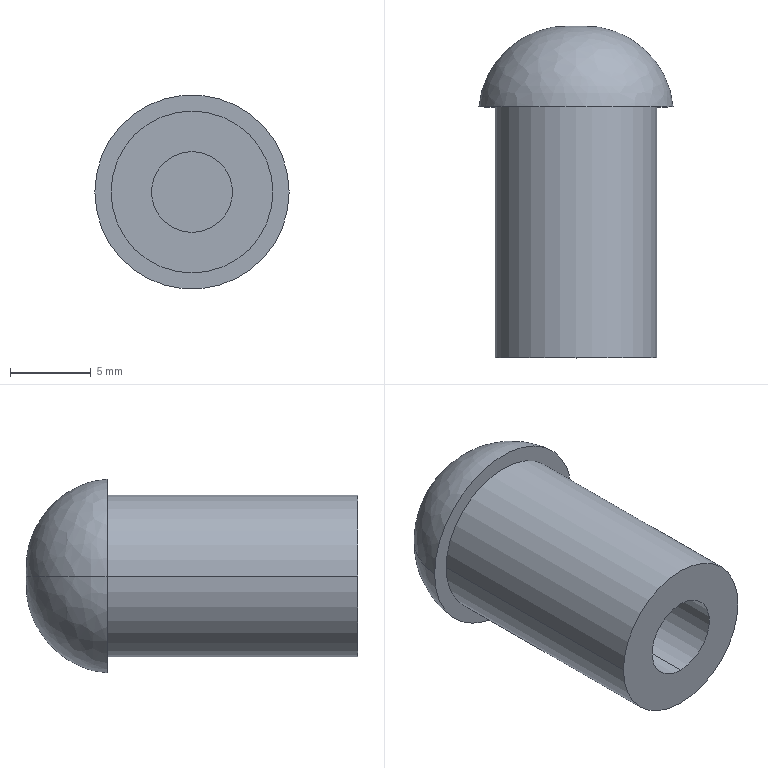Part | STEP file | YELUNDUTOU_8_1 | 1 solid | 10 faces | box 12 x 20.5 x 12 mm | volume 1376 mm3 | plane 4 | cylinder 4 | spline 2 | commonest cylinder face diameters 5 x2 10 x2
STEP:
#1=CARTESIAN_POINT('',(0.,0.,0.));
#2=DIRECTION('',(0.,0.,1.));
#3=DIRECTION('',(1.,0.,0.));
#4=AXIS2_PLACEMENT_3D('',#1,#2,#3);
#5=CARTESIAN_POINT('',(5.,0.,0.));
#6=VERTEX_POINT('',#5);
#7=CARTESIAN_POINT('',(-5.,0.,0.));
#8=VERTEX_POINT('',#7);
#9=CARTESIAN_POINT('',(0.,0.,0.));
#10=DIRECTION('',(0.,1.,0.));
#11=DIRECTION('',(1.,0.,0.));
#12=AXIS2_PLACEMENT_3D('',#9,#10,#11);
#13=CIRCLE('',#12,5.);
#14=EDGE_CURVE('',#6,#8,#13,.T.);
#15=ORIENTED_EDGE('',*,*,#14,.T.);
#16=CARTESIAN_POINT('',(0.,0.,0.));
#17=DIRECTION('',(0.,1.,0.));
#18=DIRECTION('',(-1.,0.,0.));
#19=AXIS2_PLACEMENT_3D('',#16,#17,#18);
#20=CIRCLE('',#19,5.);
#21=EDGE_CURVE('',#8,#6,#20,.T.);
#22=ORIENTED_EDGE('',*,*,#21,.T.);
#23=EDGE_LOOP('',(#15,#22));
#24=FACE_OUTER_BOUND('',#23,.F.);
#25=CARTESIAN_POINT('',(0.,0.,2.5));
#26=VERTEX_POINT('',#25);
#27=CARTESIAN_POINT('',(0.,0.,-2.5));
#28=VERTEX_POINT('',#27);
#29=CARTESIAN_POINT('',(0.,0.,0.));
#30=DIRECTION('',(0.,-1.,0.));
#31=DIRECTION('',(0.,0.,1.));
#32=AXIS2_PLACEMENT_3D('',#29,#30,#31);
#33=CIRCLE('',#32,2.5);
#34=EDGE_CURVE('',#26,#28,#33,.T.);
#35=ORIENTED_EDGE('',*,*,#34,.T.);
#36=CARTESIAN_POINT('',(0.,0.,0.));
#37=DIRECTION('',(0.,-1.,0.));
#38=DIRECTION('',(0.,0.,-1.));
#39=AXIS2_PLACEMENT_3D('',#36,#37,#38);
#40=CIRCLE('',#39,2.5);
#41=EDGE_CURVE('',#28,#26,#40,.T.);
#42=ORIENTED_EDGE('',*,*,#41,.T.);
#43=EDGE_LOOP('',(#35,#42));
#44=FACE_BOUND('',#43,.F.);
#45=CARTESIAN_POINT('',(0.,0.,0.));
#46=DIRECTION('',(0.,1.,0.));
#47=DIRECTION('',(1.,0.,0.));
#48=AXIS2_PLACEMENT_3D('',#45,#46,#47);
#49=PLANE('',#48);
#50=ADVANCED_FACE('',(#24,#44),#49,.F.);
#51=CARTESIAN_POINT('',(-5.,15.5,0.));
#52=VERTEX_POINT('',#51);
#53=CARTESIAN_POINT('',(5.,15.5,0.));
#54=VERTEX_POINT('',#53);
#55=CARTESIAN_POINT('',(0.,15.5,0.));
#56=DIRECTION('',(0.,-1.,0.));
#57=DIRECTION('',(-1.,0.,0.));
#58=AXIS2_PLACEMENT_3D('',#55,#56,#57);
#59=CIRCLE('',#58,5.);
#60=EDGE_CURVE('',#52,#54,#59,.T.);
#61=ORIENTED_EDGE('',*,*,#60,.F.);
#62=CARTESIAN_POINT('',(-5.,0.,0.));
#63=DIRECTION('',(0.,1.,0.));
#64=VECTOR('',#63,15.5);
#65=LINE('',#62,#64);
#66=EDGE_CURVE('',#8,#52,#65,.T.);
#67=ORIENTED_EDGE('',*,*,#66,.F.);
#68=ORIENTED_EDGE('',*,*,#14,.F.);
#69=CARTESIAN_POINT('',(5.,0.,0.));
#70=DIRECTION('',(0.,1.,0.));
#71=VECTOR('',#70,15.5);
#72=LINE('',#69,#71);
#73=EDGE_CURVE('',#6,#54,#72,.T.);
#74=ORIENTED_EDGE('',*,*,#73,.T.);
#75=EDGE_LOOP('',(#61,#67,#68,#74));
#76=FACE_OUTER_BOUND('',#75,.F.);
#77=CARTESIAN_POINT('',(0.,0.,0.));
#78=DIRECTION('',(0.,1.,0.));
#79=DIRECTION('',(1.,0.,0.));
#80=AXIS2_PLACEMENT_3D('',#77,#78,#79);
#81=CYLINDRICAL_SURFACE('',#80,5.);
#82=ADVANCED_FACE('',(#76),#81,.T.);
#83=CARTESIAN_POINT('',(-6.,15.5,0.));
#84=VERTEX_POINT('',#83);
#85=CARTESIAN_POINT('',(6.,15.5,0.));
#86=VERTEX_POINT('',#85);
#87=CARTESIAN_POINT('',(0.,15.5,0.));
#88=DIRECTION('',(0.,1.,0.));
#89=DIRECTION('',(-1.,0.,0.));
#90=AXIS2_PLACEMENT_3D('',#87,#88,#89);
#91=CIRCLE('',#90,6.);
#92=EDGE_CURVE('',#84,#86,#91,.T.);
#93=ORIENTED_EDGE('',*,*,#92,.T.);
#94=CARTESIAN_POINT('',(0.,15.5,0.));
#95=DIRECTION('',(0.,1.,0.));
#96=DIRECTION('',(1.,0.,0.));
#97=AXIS2_PLACEMENT_3D('',#94,#95,#96);
#98=CIRCLE('',#97,6.);
#99=EDGE_CURVE('',#86,#84,#98,.T.);
#100=ORIENTED_EDGE('',*,*,#99,.T.);
#101=EDGE_LOOP('',(#93,#100));
#102=FACE_OUTER_BOUND('',#101,.F.);
#103=ORIENTED_EDGE('',*,*,#60,.T.);
#104=CARTESIAN_POINT('',(0.,15.5,0.));
#105=DIRECTION('',(0.,-1.,0.));
#106=DIRECTION('',(1.,0.,0.));
#107=AXIS2_PLACEMENT_3D('',#104,#105,#106);
#108=CIRCLE('',#107,5.);
#109=EDGE_CURVE('',#54,#52,#108,.T.);
#110=ORIENTED_EDGE('',*,*,#109,.T.);
#111=EDGE_LOOP('',(#103,#110));
#112=FACE_BOUND('',#111,.F.);
#113=CARTESIAN_POINT('',(0.,15.5,0.));
#114=DIRECTION('',(0.,1.,0.));
#115=DIRECTION('',(1.,0.,0.));
#116=AXIS2_PLACEMENT_3D('',#113,#114,#115);
#117=PLANE('',#116);
#118=ADVANCED_FACE('',(#102,#112),#117,.F.);
#119=CARTESIAN_POINT('',(0.5228,20.5,0.));
#120=VERTEX_POINT('',#119);
#121=CARTESIAN_POINT('',(-0.5228,20.5,0.));
#122=VERTEX_POINT('',#121);
#123=CARTESIAN_POINT('',(0.,20.5,0.));
#124=DIRECTION('',(0.,-1.,0.));
#125=DIRECTION('',(1.,0.,0.));
#126=AXIS2_PLACEMENT_3D('',#123,#124,#125);
#127=CIRCLE('',#126,0.5228);
#128=EDGE_CURVE('',#120,#122,#127,.T.);
#129=ORIENTED_EDGE('',*,*,#128,.F.);
#130=CARTESIAN_POINT('',(0.5228,15.,0.0000047));
#131=DIRECTION('',(0.000008991,0.,-1.));
#132=DIRECTION('',(0.000004504,1.,0.));
#133=AXIS2_PLACEMENT_3D('',#130,#131,#132);
#134=CIRCLE('',#133,5.5);
#135=EDGE_CURVE('',#120,#86,#134,.T.);
#136=ORIENTED_EDGE('',*,*,#135,.T.);
#137=ORIENTED_EDGE('',*,*,#92,.F.);
#138=CARTESIAN_POINT('',(-0.5228,15.,-0.0000047));
#139=DIRECTION('',(-0.000008991,0.,1.));
#140=DIRECTION('',(-0.000004504,1.,0.));
#141=AXIS2_PLACEMENT_3D('',#138,#139,#140);
#142=CIRCLE('',#141,5.5);
#143=EDGE_CURVE('',#122,#84,#142,.T.);
#144=ORIENTED_EDGE('',*,*,#143,.F.);
#145=EDGE_LOOP('',(#129,#136,#137,#144));
#146=FACE_OUTER_BOUND('',#145,.F.);
#147=CARTESIAN_POINT('',(-6.001,15.338,-0.3775));
#148=CARTESIAN_POINT('',(-5.808,18.473,-0.3654));
#149=CARTESIAN_POINT('',(-3.493,20.591,-0.2197));
#150=CARTESIAN_POINT('',(-0.3593,20.498,-0.0226));
#151=CARTESIAN_POINT('',(-6.233,15.338,3.315));
#152=CARTESIAN_POINT('',(-6.033,18.473,3.209));
#153=CARTESIAN_POINT('',(-3.628,20.591,1.93));
#154=CARTESIAN_POINT('',(-0.3732,20.498,0.1985));
#155=CARTESIAN_POINT('',(-3.7,15.338,6.012));
#156=CARTESIAN_POINT('',(-3.581,18.473,5.82));
#157=CARTESIAN_POINT('',(-2.154,20.591,3.5));
#158=CARTESIAN_POINT('',(-0.2216,20.498,0.36));
#159=CARTESIAN_POINT('',(0.00002964,15.338,6.012));
#160=CARTESIAN_POINT('',(0.00002869,18.473,5.82));
#161=CARTESIAN_POINT('',(0.00001725,20.591,3.5));
#162=CARTESIAN_POINT('',(0.000001775,20.498,0.36));
#163=CARTESIAN_POINT('',(3.7,15.338,6.012));
#164=CARTESIAN_POINT('',(3.581,18.473,5.819));
#165=CARTESIAN_POINT('',(2.154,20.591,3.5));
#166=CARTESIAN_POINT('',(0.2216,20.498,0.36));
#167=CARTESIAN_POINT('',(6.233,15.338,3.315));
#168=CARTESIAN_POINT('',(6.033,18.473,3.209));
#169=CARTESIAN_POINT('',(3.628,20.591,1.93));
#170=CARTESIAN_POINT('',(0.3732,20.498,0.1985));
#171=CARTESIAN_POINT('',(6.001,15.338,-0.3775));
#172=CARTESIAN_POINT('',(5.808,18.473,-0.3654));
#173=CARTESIAN_POINT('',(3.493,20.591,-0.2198));
#174=CARTESIAN_POINT('',(0.3593,20.498,-0.02261));
#175=(BOUNDED_SURFACE()B_SPLINE_SURFACE(3,3,((#147,#148,#149,#150),(#151,#152,#153,#154),(#155,#156,#157,#158),(#159,#160,#161,#162),(#163,#164,#165,#166),(#167,#168,#169,#170),(#171,#172,#173,#174)),.UNSPECIFIED.,.F.,.F.,.F.)B_SPLINE_SURFACE_WITH_KNOTS((4,3,4),(4,4),(0.,1.,2.),(0.,1.),.UNSPECIFIED.)GEOMETRIC_REPRESENTATION_ITEM()RATIONAL_B_SPLINE_SURFACE(((1.382,1.122,1.122,1.382),(1.091,0.8863,0.8863,1.091),(1.091,0.8863,0.8863,1.091),(1.382,1.122,1.122,1.382),(1.091,0.8863,0.8863,1.091),(1.091,0.8863,0.8863,1.091),(1.382,1.122,1.122,1.382)))REPRESENTATION_ITEM('')SURFACE());
#176=ADVANCED_FACE('',(#146),#175,.T.);
#177=ORIENTED_EDGE('',*,*,#128,.T.);
#178=CARTESIAN_POINT('',(0.,20.5,0.));
#179=DIRECTION('',(0.,-1.,0.));
#180=DIRECTION('',(-1.,0.,0.));
#181=AXIS2_PLACEMENT_3D('',#178,#179,#180);
#182=CIRCLE('',#181,0.5228);
#183=EDGE_CURVE('',#122,#120,#182,.T.);
#184=ORIENTED_EDGE('',*,*,#183,.T.);
#185=EDGE_LOOP('',(#177,#184));
#186=FACE_OUTER_BOUND('',#185,.F.);
#187=CARTESIAN_POINT('',(0.,20.5,0.));
#188=DIRECTION('',(0.,1.,0.));
#189=DIRECTION('',(1.,0.,0.));
#190=AXIS2_PLACEMENT_3D('',#187,#188,#189);
#191=PLANE('',#190);
#192=ADVANCED_FACE('',(#186),#191,.T.);
#193=ORIENTED_EDGE('',*,*,#183,.F.);
#194=ORIENTED_EDGE('',*,*,#143,.T.);
#195=ORIENTED_EDGE('',*,*,#99,.F.);
#196=ORIENTED_EDGE('',*,*,#135,.F.);
#197=EDGE_LOOP('',(#193,#194,#195,#196));
#198=FACE_OUTER_BOUND('',#197,.F.);
#199=CARTESIAN_POINT('',(6.001,15.338,0.3775));
#200=CARTESIAN_POINT('',(5.808,18.473,0.3654));
#201=CARTESIAN_POINT('',(3.493,20.591,0.2197));
#202=CARTESIAN_POINT('',(0.3593,20.498,0.0226));
#203=CARTESIAN_POINT('',(6.233,15.338,-3.315));
#204=CARTESIAN_POINT('',(6.033,18.473,-3.209));
#205=CARTESIAN_POINT('',(3.628,20.591,-1.93));
#206=CARTESIAN_POINT('',(0.3732,20.498,-0.1985));
#207=CARTESIAN_POINT('',(3.7,15.338,-6.012));
#208=CARTESIAN_POINT('',(3.581,18.473,-5.82));
#209=CARTESIAN_POINT('',(2.154,20.591,-3.5));
#210=CARTESIAN_POINT('',(0.2216,20.498,-0.36));
#211=CARTESIAN_POINT('',(-0.00002964,15.338,-6.012));
#212=CARTESIAN_POINT('',(-0.00002869,18.473,-5.82));
#213=CARTESIAN_POINT('',(-0.00001725,20.591,-3.5));
#214=CARTESIAN_POINT('',(-0.000001775,20.498,-0.36));
#215=CARTESIAN_POINT('',(-3.7,15.338,-6.012));
#216=CARTESIAN_POINT('',(-3.581,18.473,-5.819));
#217=CARTESIAN_POINT('',(-2.154,20.591,-3.5));
#218=CARTESIAN_POINT('',(-0.2216,20.498,-0.36));
#219=CARTESIAN_POINT('',(-6.233,15.338,-3.315));
#220=CARTESIAN_POINT('',(-6.033,18.473,-3.209));
#221=CARTESIAN_POINT('',(-3.628,20.591,-1.93));
#222=CARTESIAN_POINT('',(-0.3732,20.498,-0.1985));
#223=CARTESIAN_POINT('',(-6.001,15.338,0.3775));
#224=CARTESIAN_POINT('',(-5.808,18.473,0.3654));
#225=CARTESIAN_POINT('',(-3.493,20.591,0.2198));
#226=CARTESIAN_POINT('',(-0.3593,20.498,0.02261));
#227=(BOUNDED_SURFACE()B_SPLINE_SURFACE(3,3,((#199,#200,#201,#202),(#203,#204,#205,#206),(#207,#208,#209,#210),(#211,#212,#213,#214),(#215,#216,#217,#218),(#219,#220,#221,#222),(#223,#224,#225,#226)),.UNSPECIFIED.,.F.,.F.,.F.)B_SPLINE_SURFACE_WITH_KNOTS((4,3,4),(4,4),(0.,1.,2.),(0.,1.),.UNSPECIFIED.)GEOMETRIC_REPRESENTATION_ITEM()RATIONAL_B_SPLINE_SURFACE(((1.382,1.122,1.122,1.382),(1.091,0.8863,0.8863,1.091),(1.091,0.8863,0.8863,1.091),(1.382,1.122,1.122,1.382),(1.091,0.8863,0.8863,1.091),(1.091,0.8863,0.8863,1.091),(1.382,1.122,1.122,1.382)))REPRESENTATION_ITEM('')SURFACE());
#228=ADVANCED_FACE('',(#198),#227,.T.);
#229=ORIENTED_EDGE('',*,*,#109,.F.);
#230=ORIENTED_EDGE('',*,*,#73,.F.);
#231=ORIENTED_EDGE('',*,*,#21,.F.);
#232=ORIENTED_EDGE('',*,*,#66,.T.);
#233=EDGE_LOOP('',(#229,#230,#231,#232));
#234=FACE_OUTER_BOUND('',#233,.F.);
#235=CARTESIAN_POINT('',(0.,0.,0.));
#236=DIRECTION('',(0.,1.,0.));
#237=DIRECTION('',(1.,0.,0.));
#238=AXIS2_PLACEMENT_3D('',#235,#236,#237);
#239=CYLINDRICAL_SURFACE('',#238,5.);
#240=ADVANCED_FACE('',(#234),#239,.T.);
#241=ORIENTED_EDGE('',*,*,#34,.F.);
#242=CARTESIAN_POINT('',(0.,11.,2.5));
#243=VERTEX_POINT('',#242);
#244=CARTESIAN_POINT('',(0.,0.,2.5));
#245=DIRECTION('',(0.,1.,0.));
#246=VECTOR('',#245,11.);
#247=LINE('',#244,#246);
#248=EDGE_CURVE('',#26,#243,#247,.T.);
#249=ORIENTED_EDGE('',*,*,#248,.T.);
#250=CARTESIAN_POINT('',(0.,11.,-2.5));
#251=VERTEX_POINT('',#250);
#252=CARTESIAN_POINT('',(0.,11.,0.));
#253=DIRECTION('',(0.,1.,0.));
#254=DIRECTION('',(0.,0.,-1.));
#255=AXIS2_PLACEMENT_3D('',#252,#253,#254);
#256=CIRCLE('',#255,2.5);
#257=EDGE_CURVE('',#251,#243,#256,.T.);
#258=ORIENTED_EDGE('',*,*,#257,.F.);
#259=CARTESIAN_POINT('',(0.,0.,-2.5));
#260=DIRECTION('',(0.,1.,0.));
#261=VECTOR('',#260,11.);
#262=LINE('',#259,#261);
#263=EDGE_CURVE('',#28,#251,#262,.T.);
#264=ORIENTED_EDGE('',*,*,#263,.F.);
#265=EDGE_LOOP('',(#241,#249,#258,#264));
#266=FACE_OUTER_BOUND('',#265,.F.);
#267=CARTESIAN_POINT('',(0.,0.,0.));
#268=DIRECTION('',(0.,-1.,0.));
#269=DIRECTION('',(0.,0.,1.));
#270=AXIS2_PLACEMENT_3D('',#267,#268,#269);
#271=CYLINDRICAL_SURFACE('',#270,2.5);
#272=ADVANCED_FACE('',(#266),#271,.F.);
#273=ORIENTED_EDGE('',*,*,#41,.F.);
#274=ORIENTED_EDGE('',*,*,#263,.T.);
#275=CARTESIAN_POINT('',(0.,11.,0.));
#276=DIRECTION('',(0.,1.,0.));
#277=DIRECTION('',(0.,0.,1.));
#278=AXIS2_PLACEMENT_3D('',#275,#276,#277);
#279=CIRCLE('',#278,2.5);
#280=EDGE_CURVE('',#243,#251,#279,.T.);
#281=ORIENTED_EDGE('',*,*,#280,.F.);
#282=ORIENTED_EDGE('',*,*,#248,.F.);
#283=EDGE_LOOP('',(#273,#274,#281,#282));
#284=FACE_OUTER_BOUND('',#283,.F.);
#285=CARTESIAN_POINT('',(0.,0.,0.));
#286=DIRECTION('',(0.,-1.,0.));
#287=DIRECTION('',(0.,0.,1.));
#288=AXIS2_PLACEMENT_3D('',#285,#286,#287);
#289=CYLINDRICAL_SURFACE('',#288,2.5);
#290=ADVANCED_FACE('',(#284),#289,.F.);
#291=ORIENTED_EDGE('',*,*,#257,.T.);
#292=ORIENTED_EDGE('',*,*,#280,.T.);
#293=EDGE_LOOP('',(#291,#292));
#294=FACE_OUTER_BOUND('',#293,.F.);
#295=CARTESIAN_POINT('',(0.,11.,0.));
#296=DIRECTION('',(0.,-1.,0.));
#297=DIRECTION('',(0.,0.,1.));
#298=AXIS2_PLACEMENT_3D('',#295,#296,#297);
#299=PLANE('',#298);
#300=ADVANCED_FACE('',(#294),#299,.T.);
#301=CLOSED_SHELL('',(#50,#82,#118,#176,#192,#228,#240,#272,#290,#300));
#302=MANIFOLD_SOLID_BREP('',#301);
#303=(LENGTH_UNIT()NAMED_UNIT(*)SI_UNIT(.MILLI.,.METRE.));
#304=UNCERTAINTY_MEASURE_WITH_UNIT(LENGTH_MEASURE(0.002662),#303,'','');
#305=(NAMED_UNIT(*)PLANE_ANGLE_UNIT()SI_UNIT($,.RADIAN.));
#306=PLANE_ANGLE_MEASURE_WITH_UNIT(PLANE_ANGLE_MEASURE(0.01745),#305);
#307=(CONVERSION_BASED_UNIT('DEGREE',#306)NAMED_UNIT(*)PLANE_ANGLE_UNIT());
#308=(NAMED_UNIT(*)SI_UNIT($,.STERADIAN.)SOLID_ANGLE_UNIT());
#309=(GEOMETRIC_REPRESENTATION_CONTEXT(3)GLOBAL_UNCERTAINTY_ASSIGNED_CONTEXT((#304))GLOBAL_UNIT_ASSIGNED_CONTEXT((#303,#307,#308))REPRESENTATION_CONTEXT('',''));
#310=ADVANCED_BREP_SHAPE_REPRESENTATION('',(#4,#302),#309);